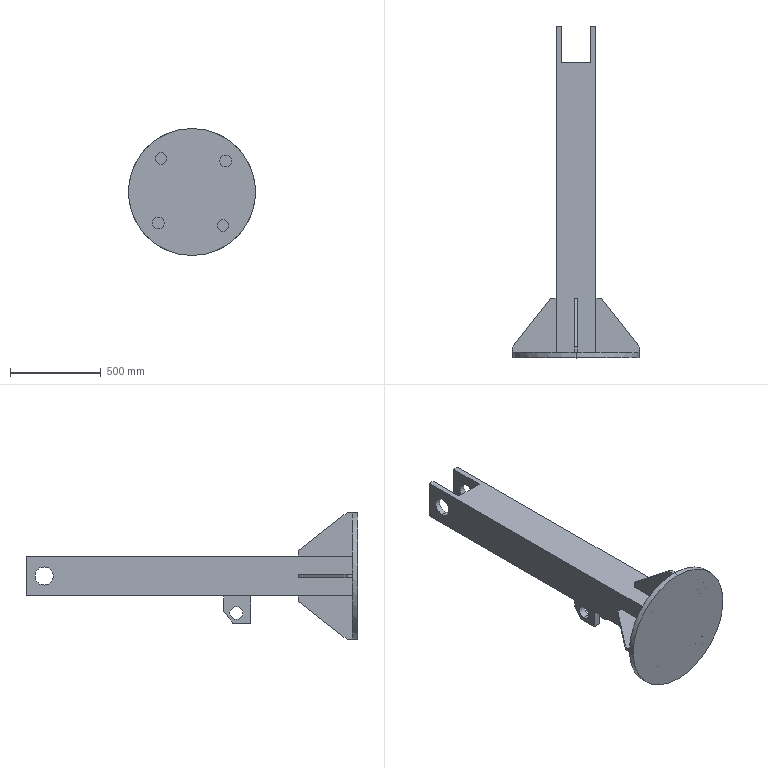Part | SolidWorks | features BaseBody 1 | 1 solid | 84 faces | box 700 x 1830 x 700 mm | volume 31659416 mm3 | plane 66 | cylinder 18 | commonest cylinder face diameters 65 x8 72 x4 100 x4 700 x2